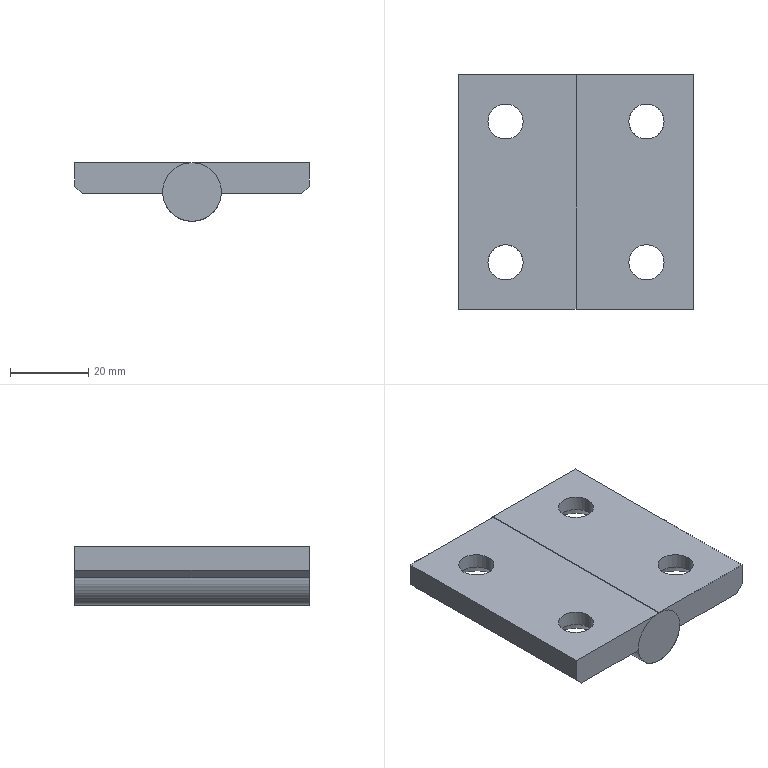Part | SolidWorks | 2 solids | 32 faces | box 60 x 60 x 15 mm | volume 40706 mm3 | cylinder 12 | plane 12 | cone 8 | commonest cylinder face diameters 9 x8 15 x4